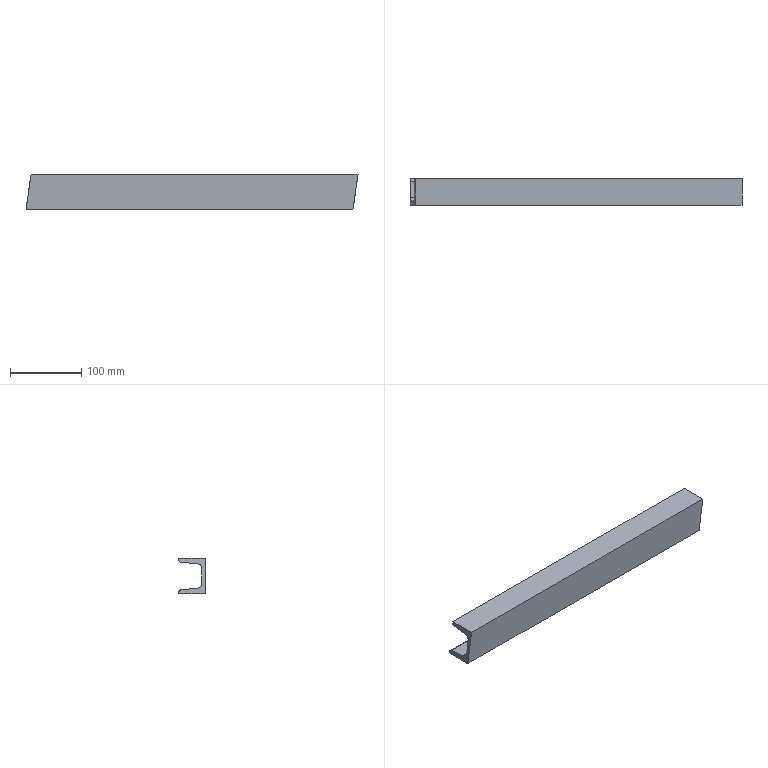Part | SolidWorks | features ICE 1, WeldMemberFeat 1, WeldmentFeature 1 | 1 solid | 14 faces | box 465.489 x 37 x 50 mm | volume 317394 mm3 | plane 10 | cylinder 4 | commonest cylinder face diameters 7 x2 14 x2
STEP:
#1=CARTESIAN_POINT('',(-35.301,33.866,44.379));
#2=VERTEX_POINT('',#1);
#3=CARTESIAN_POINT('',(-493.763,33.866,44.379));
#4=VERTEX_POINT('',#3);
#5=CARTESIAN_POINT('',(500.,33.866,44.379));
#6=DIRECTION('',(-1.,0.,0.));
#7=VECTOR('',#6,1000.);
#8=LINE('',#5,#7);
#9=EDGE_CURVE('',#2,#4,#8,.T.);
#10=ORIENTED_EDGE('',*,*,#9,.T.);
#11=CARTESIAN_POINT('',(-493.274,37.,47.859));
#12=VERTEX_POINT('',#11);
#13=CARTESIAN_POINT('',(-493.763,33.866,44.379));
#14=CARTESIAN_POINT('',(-493.735,35.739,44.575));
#15=CARTESIAN_POINT('',(-493.539,37.,45.975));
#16=CARTESIAN_POINT('',(-493.274,37.,47.859));
#17=(BOUNDED_CURVE()B_SPLINE_CURVE(3,(#13,#14,#15,#16),.UNSPECIFIED.,.F.,.F.)B_SPLINE_CURVE_WITH_KNOTS((4,4),(0.1047,1.571),.UNSPECIFIED.)CURVE()GEOMETRIC_REPRESENTATION_ITEM()RATIONAL_B_SPLINE_CURVE((1.,0.8288,0.8288,1.))REPRESENTATION_ITEM(''));
#18=EDGE_CURVE('',#4,#12,#17,.T.);
#19=ORIENTED_EDGE('',*,*,#18,.T.);
#20=CARTESIAN_POINT('',(-34.812,37.,47.859));
#21=VERTEX_POINT('',#20);
#22=CARTESIAN_POINT('',(500.,37.,47.859));
#23=DIRECTION('',(-1.,0.,0.));
#24=VECTOR('',#23,1000.);
#25=LINE('',#22,#24);
#26=EDGE_CURVE('',#21,#12,#25,.T.);
#27=ORIENTED_EDGE('',*,*,#26,.F.);
#28=CARTESIAN_POINT('',(-34.812,37.,47.859));
#29=CARTESIAN_POINT('',(-35.077,37.,45.975));
#30=CARTESIAN_POINT('',(-35.274,35.739,44.575));
#31=CARTESIAN_POINT('',(-35.301,33.866,44.379));
#32=(BOUNDED_CURVE()B_SPLINE_CURVE(3,(#28,#29,#30,#31),.UNSPECIFIED.,.F.,.F.)B_SPLINE_CURVE_WITH_KNOTS((4,4),(4.712,6.178),.UNSPECIFIED.)CURVE()GEOMETRIC_REPRESENTATION_ITEM()RATIONAL_B_SPLINE_CURVE((1.,0.8288,0.8288,1.))REPRESENTATION_ITEM(''));
#33=EDGE_CURVE('',#21,#2,#32,.T.);
#34=ORIENTED_EDGE('',*,*,#33,.T.);
#35=EDGE_LOOP('',(#10,#19,#27,#34));
#36=FACE_OUTER_BOUND('',#35,.T.);
#37=CARTESIAN_POINT('',(500.,33.5,47.859));
#38=DIRECTION('',(-1.,0.,0.));
#39=DIRECTION('',(0.,-1.,0.));
#40=AXIS2_PLACEMENT_3D('',#37,#38,#39);
#41=CYLINDRICAL_SURFACE('',#40,3.5);
#42=ADVANCED_FACE('',(#36),#41,.T.);
#43=ORIENTED_EDGE('',*,*,#26,.T.);
#44=CARTESIAN_POINT('',(-492.973,37.,50.));
#45=VERTEX_POINT('',#44);
#46=CARTESIAN_POINT('',(-500.,37.,0.));
#47=DIRECTION('',(0.1392,0.,0.9903));
#48=VECTOR('',#47,1000.);
#49=LINE('',#46,#48);
#50=EDGE_CURVE('',#12,#45,#49,.T.);
#51=ORIENTED_EDGE('',*,*,#50,.T.);
#52=CARTESIAN_POINT('',(-34.511,37.,50.));
#53=VERTEX_POINT('',#52);
#54=CARTESIAN_POINT('',(500.,37.,50.));
#55=DIRECTION('',(-1.,0.,0.));
#56=VECTOR('',#55,1000.);
#57=LINE('',#54,#56);
#58=EDGE_CURVE('',#53,#45,#57,.T.);
#59=ORIENTED_EDGE('',*,*,#58,.F.);
#60=CARTESIAN_POINT('',(-34.511,37.,50.));
#61=DIRECTION('',(-0.1392,0.,-0.9903));
#62=VECTOR('',#61,1000.);
#63=LINE('',#60,#62);
#64=EDGE_CURVE('',#53,#21,#63,.T.);
#65=ORIENTED_EDGE('',*,*,#64,.T.);
#66=EDGE_LOOP('',(#43,#51,#59,#65));
#67=FACE_OUTER_BOUND('',#66,.T.);
#68=CARTESIAN_POINT('',(500.,37.,50.));
#69=DIRECTION('',(0.,-1.,0.));
#70=DIRECTION('',(1.,0.,0.));
#71=AXIS2_PLACEMENT_3D('',#68,#69,#70);
#72=PLANE('',#71);
#73=ADVANCED_FACE('',(#67),#72,.F.);
#74=ORIENTED_EDGE('',*,*,#58,.T.);
#75=CARTESIAN_POINT('',(-492.973,0.,50.));
#76=VERTEX_POINT('',#75);
#77=CARTESIAN_POINT('',(-492.973,37.,50.));
#78=DIRECTION('',(0.,-1.,0.));
#79=VECTOR('',#78,1000.);
#80=LINE('',#77,#79);
#81=EDGE_CURVE('',#45,#76,#80,.T.);
#82=ORIENTED_EDGE('',*,*,#81,.T.);
#83=CARTESIAN_POINT('',(-34.511,0.,50.));
#84=VERTEX_POINT('',#83);
#85=CARTESIAN_POINT('',(500.,0.,50.));
#86=DIRECTION('',(-1.,0.,0.));
#87=VECTOR('',#86,1000.);
#88=LINE('',#85,#87);
#89=EDGE_CURVE('',#84,#76,#88,.T.);
#90=ORIENTED_EDGE('',*,*,#89,.F.);
#91=CARTESIAN_POINT('',(-34.511,37.,50.));
#92=DIRECTION('',(0.,-1.,0.));
#93=VECTOR('',#92,1000.);
#94=LINE('',#91,#93);
#95=EDGE_CURVE('',#53,#84,#94,.T.);
#96=ORIENTED_EDGE('',*,*,#95,.F.);
#97=EDGE_LOOP('',(#74,#82,#90,#96));
#98=FACE_OUTER_BOUND('',#97,.T.);
#99=CARTESIAN_POINT('',(500.,37.,50.));
#100=DIRECTION('',(0.,0.,-1.));
#101=DIRECTION('',(0.,1.,0.));
#102=AXIS2_PLACEMENT_3D('',#99,#100,#101);
#103=PLANE('',#102);
#104=ADVANCED_FACE('',(#98),#103,.F.);
#105=ORIENTED_EDGE('',*,*,#89,.T.);
#106=CARTESIAN_POINT('',(-500.,0.,0.));
#107=VERTEX_POINT('',#106);
#108=CARTESIAN_POINT('',(-473.74,0.,186.85));
#109=DIRECTION('',(-0.1392,0.,-0.9903));
#110=VECTOR('',#109,1000.);
#111=LINE('',#108,#110);
#112=EDGE_CURVE('',#76,#107,#111,.T.);
#113=ORIENTED_EDGE('',*,*,#112,.T.);
#114=CARTESIAN_POINT('',(-41.538,0.,0.));
#115=VERTEX_POINT('',#114);
#116=CARTESIAN_POINT('',(500.,0.,0.));
#117=DIRECTION('',(-1.,0.,0.));
#118=VECTOR('',#117,1000.);
#119=LINE('',#116,#118);
#120=EDGE_CURVE('',#115,#107,#119,.T.);
#121=ORIENTED_EDGE('',*,*,#120,.F.);
#122=CARTESIAN_POINT('',(-24.158,0.,123.666));
#123=DIRECTION('',(0.1392,0.,0.9903));
#124=VECTOR('',#123,1000.);
#125=LINE('',#122,#124);
#126=EDGE_CURVE('',#115,#84,#125,.T.);
#127=ORIENTED_EDGE('',*,*,#126,.T.);
#128=EDGE_LOOP('',(#105,#113,#121,#127));
#129=FACE_OUTER_BOUND('',#128,.T.);
#130=CARTESIAN_POINT('',(500.,0.,50.));
#131=DIRECTION('',(0.,1.,0.));
#132=DIRECTION('',(-1.,0.,0.));
#133=AXIS2_PLACEMENT_3D('',#130,#131,#132);
#134=PLANE('',#133);
#135=ADVANCED_FACE('',(#129),#134,.F.);
#136=CARTESIAN_POINT('',(-41.538,37.,0.));
#137=VERTEX_POINT('',#136);
#138=CARTESIAN_POINT('',(-500.,37.,0.));
#139=VERTEX_POINT('',#138);
#140=CARTESIAN_POINT('',(500.,37.,0.));
#141=DIRECTION('',(-1.,0.,0.));
#142=VECTOR('',#141,1000.);
#143=LINE('',#140,#142);
#144=EDGE_CURVE('',#137,#139,#143,.T.);
#145=ORIENTED_EDGE('',*,*,#144,.F.);
#146=CARTESIAN_POINT('',(-41.538,37.,0.));
#147=DIRECTION('',(0.,-1.,0.));
#148=VECTOR('',#147,1000.);
#149=LINE('',#146,#148);
#150=EDGE_CURVE('',#137,#115,#149,.T.);
#151=ORIENTED_EDGE('',*,*,#150,.T.);
#152=ORIENTED_EDGE('',*,*,#120,.T.);
#153=CARTESIAN_POINT('',(-500.,37.,0.));
#154=DIRECTION('',(0.,1.,0.));
#155=VECTOR('',#154,1000.);
#156=LINE('',#153,#155);
#157=EDGE_CURVE('',#107,#139,#156,.T.);
#158=ORIENTED_EDGE('',*,*,#157,.T.);
#159=EDGE_LOOP('',(#145,#151,#152,#158));
#160=FACE_OUTER_BOUND('',#159,.T.);
#161=CARTESIAN_POINT('',(500.,37.,0.));
#162=DIRECTION('',(0.,0.,1.));
#163=DIRECTION('',(0.,-1.,0.));
#164=AXIS2_PLACEMENT_3D('',#161,#162,#163);
#165=PLANE('',#164);
#166=ADVANCED_FACE('',(#160),#165,.F.);
#167=ORIENTED_EDGE('',*,*,#144,.T.);
#168=CARTESIAN_POINT('',(-499.699,37.,2.141));
#169=VERTEX_POINT('',#168);
#170=CARTESIAN_POINT('',(-500.,37.,0.));
#171=DIRECTION('',(0.1392,0.,0.9903));
#172=VECTOR('',#171,1000.);
#173=LINE('',#170,#172);
#174=EDGE_CURVE('',#139,#169,#173,.T.);
#175=ORIENTED_EDGE('',*,*,#174,.T.);
#176=CARTESIAN_POINT('',(-41.237,37.,2.141));
#177=VERTEX_POINT('',#176);
#178=CARTESIAN_POINT('',(500.,37.,2.141));
#179=DIRECTION('',(-1.,0.,0.));
#180=VECTOR('',#179,1000.);
#181=LINE('',#178,#180);
#182=EDGE_CURVE('',#177,#169,#181,.T.);
#183=ORIENTED_EDGE('',*,*,#182,.F.);
#184=CARTESIAN_POINT('',(-34.511,37.,50.));
#185=DIRECTION('',(-0.1392,0.,-0.9903));
#186=VECTOR('',#185,1000.);
#187=LINE('',#184,#186);
#188=EDGE_CURVE('',#177,#137,#187,.T.);
#189=ORIENTED_EDGE('',*,*,#188,.T.);
#190=EDGE_LOOP('',(#167,#175,#183,#189));
#191=FACE_OUTER_BOUND('',#190,.T.);
#192=CARTESIAN_POINT('',(500.,37.,0.));
#193=DIRECTION('',(0.,-1.,0.));
#194=DIRECTION('',(1.,0.,0.));
#195=AXIS2_PLACEMENT_3D('',#192,#193,#194);
#196=PLANE('',#195);
#197=ADVANCED_FACE('',(#191),#196,.F.);
#198=ORIENTED_EDGE('',*,*,#182,.T.);
#199=CARTESIAN_POINT('',(-499.21,33.866,5.621));
#200=VERTEX_POINT('',#199);
#201=CARTESIAN_POINT('',(-499.699,37.,2.141));
#202=CARTESIAN_POINT('',(-499.434,37.,4.025));
#203=CARTESIAN_POINT('',(-499.238,35.739,5.425));
#204=CARTESIAN_POINT('',(-499.21,33.866,5.621));
#205=(BOUNDED_CURVE()B_SPLINE_CURVE(3,(#201,#202,#203,#204),.UNSPECIFIED.,.F.,.F.)B_SPLINE_CURVE_WITH_KNOTS((4,4),(1.571,3.037),.UNSPECIFIED.)CURVE()GEOMETRIC_REPRESENTATION_ITEM()RATIONAL_B_SPLINE_CURVE((1.,0.8288,0.8288,1.))REPRESENTATION_ITEM(''));
#206=EDGE_CURVE('',#169,#200,#205,.T.);
#207=ORIENTED_EDGE('',*,*,#206,.T.);
#208=CARTESIAN_POINT('',(-40.748,33.866,5.621));
#209=VERTEX_POINT('',#208);
#210=CARTESIAN_POINT('',(500.,33.866,5.621));
#211=DIRECTION('',(-1.,0.,0.));
#212=VECTOR('',#211,1000.);
#213=LINE('',#210,#212);
#214=EDGE_CURVE('',#209,#200,#213,.T.);
#215=ORIENTED_EDGE('',*,*,#214,.F.);
#216=CARTESIAN_POINT('',(-40.748,33.866,5.621));
#217=CARTESIAN_POINT('',(-40.776,35.739,5.425));
#218=CARTESIAN_POINT('',(-40.973,37.,4.025));
#219=CARTESIAN_POINT('',(-41.237,37.,2.141));
#220=(BOUNDED_CURVE()B_SPLINE_CURVE(3,(#216,#217,#218,#219),.UNSPECIFIED.,.F.,.F.)B_SPLINE_CURVE_WITH_KNOTS((4,4),(3.246,4.712),.UNSPECIFIED.)CURVE()GEOMETRIC_REPRESENTATION_ITEM()RATIONAL_B_SPLINE_CURVE((1.,0.8288,0.8288,1.))REPRESENTATION_ITEM(''));
#221=EDGE_CURVE('',#209,#177,#220,.T.);
#222=ORIENTED_EDGE('',*,*,#221,.T.);
#223=EDGE_LOOP('',(#198,#207,#215,#222));
#224=FACE_OUTER_BOUND('',#223,.T.);
#225=CARTESIAN_POINT('',(500.,33.5,2.141));
#226=DIRECTION('',(-1.,0.,0.));
#227=DIRECTION('',(0.,-1.,0.));
#228=AXIS2_PLACEMENT_3D('',#225,#226,#227);
#229=CYLINDRICAL_SURFACE('',#228,3.5);
#230=ADVANCED_FACE('',(#224),#229,.T.);
#231=ORIENTED_EDGE('',*,*,#214,.T.);
#232=CARTESIAN_POINT('',(-498.869,10.768,8.049));
#233=VERTEX_POINT('',#232);
#234=CARTESIAN_POINT('',(-498.653,-3.822,9.583));
#235=DIRECTION('',(0.01469,-0.9944,0.1045));
#236=VECTOR('',#235,1000.);
#237=LINE('',#234,#236);
#238=EDGE_CURVE('',#200,#233,#237,.T.);
#239=ORIENTED_EDGE('',*,*,#238,.T.);
#240=CARTESIAN_POINT('',(-40.407,10.768,8.049));
#241=VERTEX_POINT('',#240);
#242=CARTESIAN_POINT('',(500.,10.768,8.049));
#243=DIRECTION('',(-1.,0.,0.));
#244=VECTOR('',#243,1000.);
#245=LINE('',#242,#244);
#246=EDGE_CURVE('',#241,#233,#245,.T.);
#247=ORIENTED_EDGE('',*,*,#246,.F.);
#248=CARTESIAN_POINT('',(-40.29,2.875,8.879));
#249=DIRECTION('',(-0.01469,0.9944,-0.1045));
#250=VECTOR('',#249,1000.);
#251=LINE('',#248,#250);
#252=EDGE_CURVE('',#241,#209,#251,.T.);
#253=ORIENTED_EDGE('',*,*,#252,.T.);
#254=EDGE_LOOP('',(#231,#239,#247,#253));
#255=FACE_OUTER_BOUND('',#254,.T.);
#256=CARTESIAN_POINT('',(500.,10.768,8.049));
#257=DIRECTION('',(0.,-0.1045,-0.9945));
#258=DIRECTION('',(0.,0.9945,-0.1045));
#259=AXIS2_PLACEMENT_3D('',#256,#257,#258);
#260=PLANE('',#259);
#261=ADVANCED_FACE('',(#255),#260,.F.);
#262=ORIENTED_EDGE('',*,*,#246,.T.);
#263=CARTESIAN_POINT('',(-497.89,4.5,15.011));
#264=VERTEX_POINT('',#263);
#265=CARTESIAN_POINT('',(-498.869,10.768,8.049));
#266=CARTESIAN_POINT('',(-498.813,7.021,8.443));
#267=CARTESIAN_POINT('',(-498.42,4.5,11.243));
#268=CARTESIAN_POINT('',(-497.89,4.5,15.011));
#269=(BOUNDED_CURVE()B_SPLINE_CURVE(3,(#265,#266,#267,#268),.UNSPECIFIED.,.F.,.T.)B_SPLINE_CURVE_WITH_KNOTS((4,4),(0.1047,1.571),.UNSPECIFIED.)CURVE()GEOMETRIC_REPRESENTATION_ITEM()RATIONAL_B_SPLINE_CURVE((1.,0.8288,0.8288,1.))REPRESENTATION_ITEM(''));
#270=EDGE_CURVE('',#233,#264,#269,.T.);
#271=ORIENTED_EDGE('',*,*,#270,.T.);
#272=CARTESIAN_POINT('',(-39.429,4.5,15.011));
#273=VERTEX_POINT('',#272);
#274=CARTESIAN_POINT('',(500.,4.5,15.011));
#275=DIRECTION('',(-1.,0.,0.));
#276=VECTOR('',#275,1000.);
#277=LINE('',#274,#276);
#278=EDGE_CURVE('',#273,#264,#277,.T.);
#279=ORIENTED_EDGE('',*,*,#278,.F.);
#280=CARTESIAN_POINT('',(-39.429,4.5,15.011));
#281=CARTESIAN_POINT('',(-39.958,4.5,11.243));
#282=CARTESIAN_POINT('',(-40.352,7.021,8.443));
#283=CARTESIAN_POINT('',(-40.407,10.768,8.049));
#284=(BOUNDED_CURVE()B_SPLINE_CURVE(3,(#280,#281,#282,#283),.UNSPECIFIED.,.F.,.T.)B_SPLINE_CURVE_WITH_KNOTS((4,4),(4.712,6.178),.UNSPECIFIED.)CURVE()GEOMETRIC_REPRESENTATION_ITEM()RATIONAL_B_SPLINE_CURVE((1.,0.8288,0.8288,1.))REPRESENTATION_ITEM(''));
#285=EDGE_CURVE('',#273,#241,#284,.T.);
#286=ORIENTED_EDGE('',*,*,#285,.T.);
#287=EDGE_LOOP('',(#262,#271,#279,#286));
#288=FACE_OUTER_BOUND('',#287,.T.);
#289=CARTESIAN_POINT('',(500.,11.5,15.011));
#290=DIRECTION('',(-1.,0.,0.));
#291=DIRECTION('',(0.,-1.,0.));
#292=AXIS2_PLACEMENT_3D('',#289,#290,#291);
#293=CYLINDRICAL_SURFACE('',#292,7.);
#294=ADVANCED_FACE('',(#288),#293,.F.);
#295=ORIENTED_EDGE('',*,*,#278,.T.);
#296=CARTESIAN_POINT('',(-495.083,4.5,34.989));
#297=VERTEX_POINT('',#296);
#298=CARTESIAN_POINT('',(-475.809,4.5,172.13));
#299=DIRECTION('',(0.1392,0.,0.9903));
#300=VECTOR('',#299,1000.);
#301=LINE('',#298,#300);
#302=EDGE_CURVE('',#264,#297,#301,.T.);
#303=ORIENTED_EDGE('',*,*,#302,.T.);
#304=CARTESIAN_POINT('',(-36.621,4.5,34.989));
#305=VERTEX_POINT('',#304);
#306=CARTESIAN_POINT('',(500.,4.5,34.989));
#307=DIRECTION('',(-1.,0.,0.));
#308=VECTOR('',#307,1000.);
#309=LINE('',#306,#308);
#310=EDGE_CURVE('',#305,#297,#309,.T.);
#311=ORIENTED_EDGE('',*,*,#310,.F.);
#312=CARTESIAN_POINT('',(-26.227,4.5,108.946));
#313=DIRECTION('',(-0.1392,0.,-0.9903));
#314=VECTOR('',#313,1000.);
#315=LINE('',#312,#314);
#316=EDGE_CURVE('',#305,#273,#315,.T.);
#317=ORIENTED_EDGE('',*,*,#316,.T.);
#318=EDGE_LOOP('',(#295,#303,#311,#317));
#319=FACE_OUTER_BOUND('',#318,.T.);
#320=CARTESIAN_POINT('',(500.,4.5,34.989));
#321=DIRECTION('',(0.,-1.,0.));
#322=DIRECTION('',(1.,0.,0.));
#323=AXIS2_PLACEMENT_3D('',#320,#321,#322);
#324=PLANE('',#323);
#325=ADVANCED_FACE('',(#319),#324,.F.);
#326=ORIENTED_EDGE('',*,*,#310,.T.);
#327=CARTESIAN_POINT('',(-494.104,10.768,41.951));
#328=VERTEX_POINT('',#327);
#329=CARTESIAN_POINT('',(-495.083,4.5,34.989));
#330=CARTESIAN_POINT('',(-494.553,4.5,38.757));
#331=CARTESIAN_POINT('',(-494.16,7.021,41.557));
#332=CARTESIAN_POINT('',(-494.104,10.768,41.951));
#333=(BOUNDED_CURVE()B_SPLINE_CURVE(3,(#329,#330,#331,#332),.UNSPECIFIED.,.F.,.F.)B_SPLINE_CURVE_WITH_KNOTS((4,4),(1.571,3.037),.UNSPECIFIED.)CURVE()GEOMETRIC_REPRESENTATION_ITEM()RATIONAL_B_SPLINE_CURVE((1.,0.8288,0.8288,1.))REPRESENTATION_ITEM(''));
#334=EDGE_CURVE('',#297,#328,#333,.T.);
#335=ORIENTED_EDGE('',*,*,#334,.T.);
#336=CARTESIAN_POINT('',(-35.642,10.768,41.951));
#337=VERTEX_POINT('',#336);
#338=CARTESIAN_POINT('',(500.,10.768,41.951));
#339=DIRECTION('',(-1.,0.,0.));
#340=VECTOR('',#339,1000.);
#341=LINE('',#338,#340);
#342=EDGE_CURVE('',#337,#328,#341,.T.);
#343=ORIENTED_EDGE('',*,*,#342,.F.);
#344=CARTESIAN_POINT('',(-35.642,10.768,41.951));
#345=CARTESIAN_POINT('',(-35.698,7.021,41.557));
#346=CARTESIAN_POINT('',(-36.091,4.5,38.757));
#347=CARTESIAN_POINT('',(-36.621,4.5,34.989));
#348=(BOUNDED_CURVE()B_SPLINE_CURVE(3,(#344,#345,#346,#347),.UNSPECIFIED.,.F.,.F.)B_SPLINE_CURVE_WITH_KNOTS((4,4),(3.246,4.712),.UNSPECIFIED.)CURVE()GEOMETRIC_REPRESENTATION_ITEM()RATIONAL_B_SPLINE_CURVE((1.,0.8288,0.8288,1.))REPRESENTATION_ITEM(''));
#349=EDGE_CURVE('',#337,#305,#348,.T.);
#350=ORIENTED_EDGE('',*,*,#349,.T.);
#351=EDGE_LOOP('',(#326,#335,#343,#350));
#352=FACE_OUTER_BOUND('',#351,.T.);
#353=CARTESIAN_POINT('',(500.,11.5,34.989));
#354=DIRECTION('',(-1.,0.,0.));
#355=DIRECTION('',(0.,-1.,0.));
#356=AXIS2_PLACEMENT_3D('',#353,#354,#355);
#357=CYLINDRICAL_SURFACE('',#356,7.);
#358=ADVANCED_FACE('',(#352),#357,.F.);
#359=ORIENTED_EDGE('',*,*,#342,.T.);
#360=CARTESIAN_POINT('',(-493.89,25.289,43.477));
#361=DIRECTION('',(0.01469,0.9944,0.1045));
#362=VECTOR('',#361,1000.);
#363=LINE('',#360,#362);
#364=EDGE_CURVE('',#328,#4,#363,.T.);
#365=ORIENTED_EDGE('',*,*,#364,.T.);
#366=ORIENTED_EDGE('',*,*,#9,.F.);
#367=CARTESIAN_POINT('',(-35.527,18.592,42.773));
#368=DIRECTION('',(-0.01469,-0.9944,-0.1045));
#369=VECTOR('',#368,1000.);
#370=LINE('',#367,#369);
#371=EDGE_CURVE('',#2,#337,#370,.T.);
#372=ORIENTED_EDGE('',*,*,#371,.T.);
#373=EDGE_LOOP('',(#359,#365,#366,#372));
#374=FACE_OUTER_BOUND('',#373,.T.);
#375=CARTESIAN_POINT('',(500.,10.768,41.951));
#376=DIRECTION('',(0.,-0.1045,0.9945));
#377=DIRECTION('',(0.,-0.9945,-0.1045));
#378=AXIS2_PLACEMENT_3D('',#375,#376,#377);
#379=PLANE('',#378);
#380=ADVANCED_FACE('',(#374),#379,.F.);
#381=ORIENTED_EDGE('',*,*,#81,.F.);
#382=ORIENTED_EDGE('',*,*,#50,.F.);
#383=ORIENTED_EDGE('',*,*,#18,.F.);
#384=ORIENTED_EDGE('',*,*,#364,.F.);
#385=ORIENTED_EDGE('',*,*,#334,.F.);
#386=ORIENTED_EDGE('',*,*,#302,.F.);
#387=ORIENTED_EDGE('',*,*,#270,.F.);
#388=ORIENTED_EDGE('',*,*,#238,.F.);
#389=ORIENTED_EDGE('',*,*,#206,.F.);
#390=ORIENTED_EDGE('',*,*,#174,.F.);
#391=ORIENTED_EDGE('',*,*,#157,.F.);
#392=ORIENTED_EDGE('',*,*,#112,.F.);
#393=EDGE_LOOP('',(#381,#382,#383,#384,#385,#386,#387,#388,#389,#390,#391,#392));
#394=FACE_OUTER_BOUND('',#393,.T.);
#395=CARTESIAN_POINT('',(-500.,37.,0.));
#396=DIRECTION('',(0.9903,0.,-0.1392));
#397=DIRECTION('',(-0.1392,0.,-0.9903));
#398=AXIS2_PLACEMENT_3D('',#395,#396,#397);
#399=PLANE('',#398);
#400=ADVANCED_FACE('',(#394),#399,.F.);
#401=ORIENTED_EDGE('',*,*,#150,.F.);
#402=ORIENTED_EDGE('',*,*,#188,.F.);
#403=ORIENTED_EDGE('',*,*,#221,.F.);
#404=ORIENTED_EDGE('',*,*,#252,.F.);
#405=ORIENTED_EDGE('',*,*,#285,.F.);
#406=ORIENTED_EDGE('',*,*,#316,.F.);
#407=ORIENTED_EDGE('',*,*,#349,.F.);
#408=ORIENTED_EDGE('',*,*,#371,.F.);
#409=ORIENTED_EDGE('',*,*,#33,.F.);
#410=ORIENTED_EDGE('',*,*,#64,.F.);
#411=ORIENTED_EDGE('',*,*,#95,.T.);
#412=ORIENTED_EDGE('',*,*,#126,.F.);
#413=EDGE_LOOP('',(#401,#402,#403,#404,#405,#406,#407,#408,#409,#410,#411,#412));
#414=FACE_OUTER_BOUND('',#413,.T.);
#415=CARTESIAN_POINT('',(-34.511,37.,50.));
#416=DIRECTION('',(-0.9903,0.,0.1392));
#417=DIRECTION('',(0.1392,0.,0.9903));
#418=AXIS2_PLACEMENT_3D('',#415,#416,#417);
#419=PLANE('',#418);
#420=ADVANCED_FACE('',(#414),#419,.F.);
#421=CLOSED_SHELL('',(#42,#73,#104,#135,#166,#197,#230,#261,#294,#325,#358,#380,#400,#420));
#422=MANIFOLD_SOLID_BREP('',#421);
#423=CARTESIAN_POINT('',(0.,0.,0.));
#424=DIRECTION('',(0.,0.,1.));
#425=DIRECTION('',(1.,0.,0.));
#426=AXIS2_PLACEMENT_3D('',#423,#424,#425);
#427=(LENGTH_UNIT()NAMED_UNIT(*)SI_UNIT(.MILLI.,.METRE.));
#428=UNCERTAINTY_MEASURE_WITH_UNIT(LENGTH_MEASURE(0.00001),#427,'','');
#429=(NAMED_UNIT(*)PLANE_ANGLE_UNIT()SI_UNIT($,.RADIAN.));
#430=(NAMED_UNIT(*)SI_UNIT($,.STERADIAN.)SOLID_ANGLE_UNIT());
#431=(GEOMETRIC_REPRESENTATION_CONTEXT(3)GLOBAL_UNCERTAINTY_ASSIGNED_CONTEXT((#428))GLOBAL_UNIT_ASSIGNED_CONTEXT((#427,#429,#430))REPRESENTATION_CONTEXT('',''));
#432=ADVANCED_BREP_SHAPE_REPRESENTATION('',(#422,#426),#431);